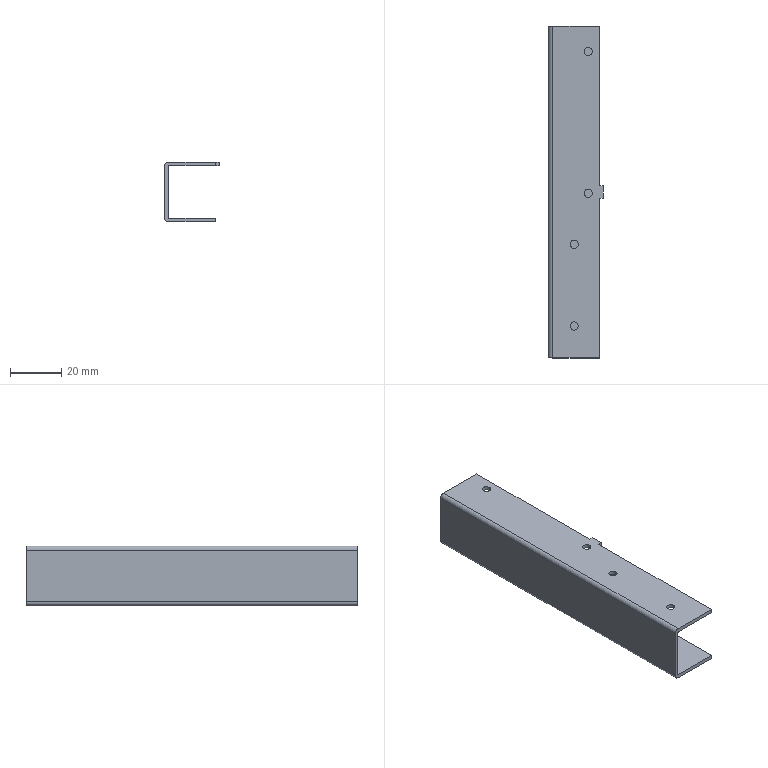Part | STEP file | HESS-408-70-15W-W-24-lower door support bracket | 1 solid | 26 faces | box 21.5 x 130 x 23.5 mm | volume 11618 mm3 | plane 14 | cylinder 12 | commonest cylinder face diameters 3.2 x10 0.2 x2